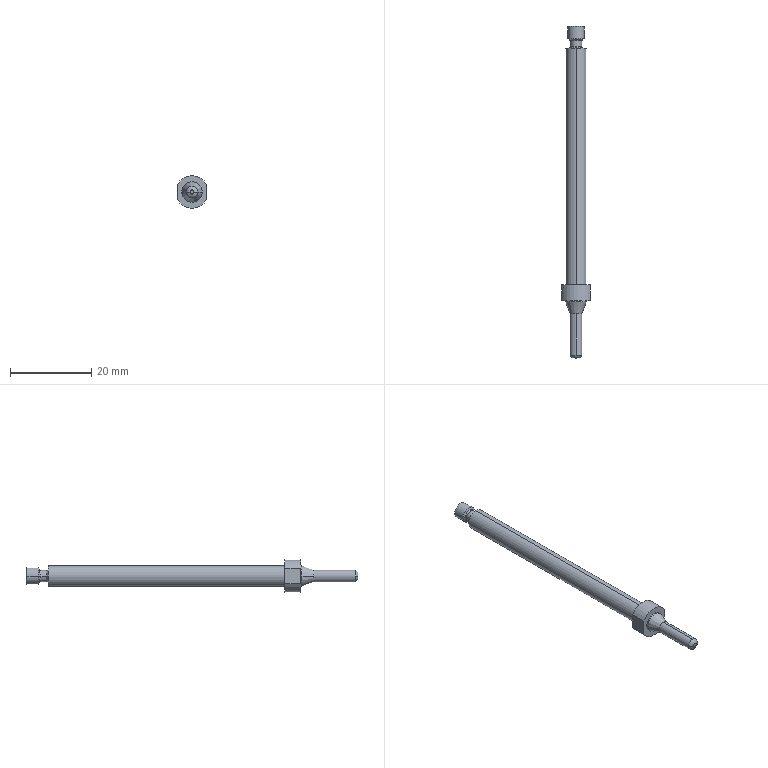Part | NX | 1 solid | 34 faces | box 7 x 81.5 x 8 mm | volume 1494 mm3 | cylinder 14 | plane 8 | cone 6 | torus 6 | commonest cylinder face diameters 4 x4 5 x4 2.8 x2 2.9 x2 8 x2
STEP:
#1=CARTESIAN_POINT('',(-125.5,76.718,117.869));
#2=VERTEX_POINT('',#1);
#3=CARTESIAN_POINT('',(-124.5,76.718,117.869));
#4=VERTEX_POINT('',#3);
#5=CARTESIAN_POINT('',(-125.,76.718,117.869));
#6=DIRECTION('',(0.,1.,0.));
#7=DIRECTION('',(0.,0.,1.));
#8=AXIS2_PLACEMENT_3D('',#5,#6,#7);
#9=CIRCLE('',#8,0.5);
#10=EDGE_CURVE('',#2,#4,#9,.T.);
#11=ORIENTED_EDGE('',*,*,#10,.F.);
#12=CARTESIAN_POINT('',(-125.,76.718,117.869));
#13=DIRECTION('',(0.,1.,0.));
#14=DIRECTION('',(0.,0.,1.));
#15=AXIS2_PLACEMENT_3D('',#12,#13,#14);
#16=CIRCLE('',#15,0.5);
#17=EDGE_CURVE('',#4,#2,#16,.T.);
#18=ORIENTED_EDGE('',*,*,#17,.F.);
#19=EDGE_LOOP('',(#11,#18));
#20=FACE_BOUND('',#19,.T.);
#21=CARTESIAN_POINT('',(-125.,76.718,119.817));
#22=DIRECTION('',(0.,1.,0.));
#23=DIRECTION('',(1.,0.,0.));
#24=AXIS2_PLACEMENT_3D('',#21,#22,#23);
#25=PLANE('',#24);
#26=ADVANCED_FACE('',(#20),#25,.F.);
#27=CARTESIAN_POINT('',(-125.,87.581,119.319));
#28=VERTEX_POINT('',#27);
#29=CARTESIAN_POINT('',(-123.55,87.581,117.869));
#30=VERTEX_POINT('',#29);
#31=CARTESIAN_POINT('',(-125.,87.581,117.869));
#32=DIRECTION('',(0.,1.,0.));
#33=DIRECTION('',(1.,0.,0.));
#34=AXIS2_PLACEMENT_3D('',#31,#32,#33);
#35=CIRCLE('',#34,1.45);
#36=EDGE_CURVE('',#28,#30,#35,.T.);
#37=ORIENTED_EDGE('',*,*,#36,.F.);
#38=CARTESIAN_POINT('',(-125.,77.406,119.319));
#39=VERTEX_POINT('',#38);
#40=CARTESIAN_POINT('',(-125.,90.3,119.319));
#41=DIRECTION('',(0.,1.,0.));
#42=VECTOR('',#41,1000.);
#43=LINE('',#40,#42);
#44=EDGE_CURVE('',#28,#39,#43,.F.);
#45=ORIENTED_EDGE('',*,*,#44,.T.);
#46=CARTESIAN_POINT('',(-123.55,77.406,117.869));
#47=VERTEX_POINT('',#46);
#48=CARTESIAN_POINT('',(-125.,77.406,117.869));
#49=DIRECTION('',(0.,1.,0.));
#50=DIRECTION('',(1.,0.,0.));
#51=AXIS2_PLACEMENT_3D('',#48,#49,#50);
#52=CIRCLE('',#51,1.45);
#53=EDGE_CURVE('',#39,#47,#52,.T.);
#54=ORIENTED_EDGE('',*,*,#53,.T.);
#55=CARTESIAN_POINT('',(-125.,77.406,116.419));
#56=VERTEX_POINT('',#55);
#57=CARTESIAN_POINT('',(-125.,77.406,117.869));
#58=DIRECTION('',(0.,1.,0.));
#59=DIRECTION('',(1.,0.,0.));
#60=AXIS2_PLACEMENT_3D('',#57,#58,#59);
#61=CIRCLE('',#60,1.45);
#62=EDGE_CURVE('',#47,#56,#61,.T.);
#63=ORIENTED_EDGE('',*,*,#62,.T.);
#64=CARTESIAN_POINT('',(-125.,87.581,116.419));
#65=VERTEX_POINT('',#64);
#66=CARTESIAN_POINT('',(-125.,90.3,116.419));
#67=DIRECTION('',(0.,1.,0.));
#68=VECTOR('',#67,1000.);
#69=LINE('',#66,#68);
#70=EDGE_CURVE('',#65,#56,#69,.F.);
#71=ORIENTED_EDGE('',*,*,#70,.F.);
#72=CARTESIAN_POINT('',(-125.,87.581,117.869));
#73=DIRECTION('',(0.,1.,0.));
#74=DIRECTION('',(1.,0.,0.));
#75=AXIS2_PLACEMENT_3D('',#72,#73,#74);
#76=CIRCLE('',#75,1.45);
#77=EDGE_CURVE('',#30,#65,#76,.T.);
#78=ORIENTED_EDGE('',*,*,#77,.F.);
#79=EDGE_LOOP('',(#37,#45,#54,#63,#71,#78));
#80=FACE_BOUND('',#79,.T.);
#81=CARTESIAN_POINT('',(-125.,90.3,117.869));
#82=DIRECTION('',(0.,1.,0.));
#83=DIRECTION('',(0.,0.,1.));
#84=AXIS2_PLACEMENT_3D('',#81,#82,#83);
#85=CYLINDRICAL_SURFACE('',#84,1.45);
#86=ADVANCED_FACE('',(#80),#85,.T.);
#87=CARTESIAN_POINT('',(-127.5,90.466,117.869));
#88=VERTEX_POINT('',#87);
#89=CARTESIAN_POINT('',(-125.,90.466,120.369));
#90=VERTEX_POINT('',#89);
#91=CARTESIAN_POINT('',(-125.,90.466,117.869));
#92=DIRECTION('',(0.,1.,0.));
#93=DIRECTION('',(0.,0.,1.));
#94=AXIS2_PLACEMENT_3D('',#91,#92,#93);
#95=CIRCLE('',#94,2.5);
#96=EDGE_CURVE('',#88,#90,#95,.T.);
#97=ORIENTED_EDGE('',*,*,#96,.F.);
#98=CARTESIAN_POINT('',(-126.45,87.581,117.869));
#99=VERTEX_POINT('',#98);
#100=CARTESIAN_POINT('',(-133.,105.577,117.869));
#101=DIRECTION('',(-0.342,0.9397,0.));
#102=VECTOR('',#101,1000.);
#103=LINE('',#100,#102);
#104=EDGE_CURVE('',#88,#99,#103,.F.);
#105=ORIENTED_EDGE('',*,*,#104,.T.);
#106=CARTESIAN_POINT('',(-125.,87.581,117.869));
#107=DIRECTION('',(0.,1.,0.));
#108=DIRECTION('',(1.,0.,0.));
#109=AXIS2_PLACEMENT_3D('',#106,#107,#108);
#110=CIRCLE('',#109,1.45);
#111=EDGE_CURVE('',#99,#28,#110,.T.);
#112=ORIENTED_EDGE('',*,*,#111,.T.);
#113=ORIENTED_EDGE('',*,*,#36,.T.);
#114=CARTESIAN_POINT('',(-122.5,90.466,117.869));
#115=VERTEX_POINT('',#114);
#116=CARTESIAN_POINT('',(-117.,105.577,117.869));
#117=DIRECTION('',(0.342,0.9397,0.));
#118=VECTOR('',#117,1000.);
#119=LINE('',#116,#118);
#120=EDGE_CURVE('',#115,#30,#119,.F.);
#121=ORIENTED_EDGE('',*,*,#120,.F.);
#122=CARTESIAN_POINT('',(-125.,90.466,117.869));
#123=DIRECTION('',(0.,1.,0.));
#124=DIRECTION('',(0.,0.,1.));
#125=AXIS2_PLACEMENT_3D('',#122,#123,#124);
#126=CIRCLE('',#125,2.5);
#127=EDGE_CURVE('',#90,#115,#126,.T.);
#128=ORIENTED_EDGE('',*,*,#127,.F.);
#129=EDGE_LOOP('',(#97,#105,#112,#113,#121,#128));
#130=FACE_BOUND('',#129,.T.);
#131=CARTESIAN_POINT('',(-125.,105.577,117.869));
#132=DIRECTION('',(0.,1.,0.));
#133=DIRECTION('',(1.,0.,0.));
#134=AXIS2_PLACEMENT_3D('',#131,#132,#133);
#135=CONICAL_SURFACE('',#134,8.,0.3491);
#136=ADVANCED_FACE('',(#130),#135,.T.);
#137=ORIENTED_EDGE('',*,*,#96,.T.);
#138=CARTESIAN_POINT('',(-125.,90.818,120.369));
#139=VERTEX_POINT('',#138);
#140=CARTESIAN_POINT('',(-125.,114.077,120.369));
#141=DIRECTION('',(0.,1.,0.));
#142=VECTOR('',#141,1000.);
#143=LINE('',#140,#142);
#144=EDGE_CURVE('',#90,#139,#143,.T.);
#145=ORIENTED_EDGE('',*,*,#144,.T.);
#146=CARTESIAN_POINT('',(-125.,90.818,115.369));
#147=VERTEX_POINT('',#146);
#148=CARTESIAN_POINT('',(-125.,90.818,117.869));
#149=DIRECTION('',(0.,1.,0.));
#150=DIRECTION('',(0.,0.,1.));
#151=AXIS2_PLACEMENT_3D('',#148,#149,#150);
#152=CIRCLE('',#151,2.5);
#153=EDGE_CURVE('',#147,#139,#152,.T.);
#154=ORIENTED_EDGE('',*,*,#153,.F.);
#155=CARTESIAN_POINT('',(-125.,90.466,115.369));
#156=VERTEX_POINT('',#155);
#157=CARTESIAN_POINT('',(-125.,114.077,115.369));
#158=DIRECTION('',(0.,1.,0.));
#159=VECTOR('',#158,1000.);
#160=LINE('',#157,#159);
#161=EDGE_CURVE('',#156,#147,#160,.T.);
#162=ORIENTED_EDGE('',*,*,#161,.F.);
#163=CARTESIAN_POINT('',(-125.,90.466,117.869));
#164=DIRECTION('',(0.,1.,0.));
#165=DIRECTION('',(0.,0.,1.));
#166=AXIS2_PLACEMENT_3D('',#163,#164,#165);
#167=CIRCLE('',#166,2.5);
#168=EDGE_CURVE('',#156,#88,#167,.T.);
#169=ORIENTED_EDGE('',*,*,#168,.T.);
#170=EDGE_LOOP('',(#137,#145,#154,#162,#169));
#171=FACE_BOUND('',#170,.T.);
#172=CARTESIAN_POINT('',(-125.,114.077,117.869));
#173=DIRECTION('',(0.,1.,0.));
#174=DIRECTION('',(0.,0.,1.));
#175=AXIS2_PLACEMENT_3D('',#172,#173,#174);
#176=CYLINDRICAL_SURFACE('',#175,2.5);
#177=ADVANCED_FACE('',(#171),#176,.T.);
#178=CARTESIAN_POINT('',(-121.5,94.718,119.805));
#179=VERTEX_POINT('',#178);
#180=CARTESIAN_POINT('',(-121.5,90.818,119.805));
#181=VERTEX_POINT('',#180);
#182=CARTESIAN_POINT('',(-121.5,94.718,119.805));
#183=DIRECTION('',(0.,-1.,0.));
#184=VECTOR('',#183,1000.);
#185=LINE('',#182,#184);
#186=EDGE_CURVE('',#179,#181,#185,.T.);
#187=ORIENTED_EDGE('',*,*,#186,.F.);
#188=CARTESIAN_POINT('',(-128.5,94.718,119.805));
#189=VERTEX_POINT('',#188);
#190=CARTESIAN_POINT('',(-125.,94.718,117.869));
#191=DIRECTION('',(0.,-1.,0.));
#192=DIRECTION('',(1.,0.,0.));
#193=AXIS2_PLACEMENT_3D('',#190,#191,#192);
#194=CIRCLE('',#193,4.);
#195=EDGE_CURVE('',#179,#189,#194,.T.);
#196=ORIENTED_EDGE('',*,*,#195,.T.);
#197=CARTESIAN_POINT('',(-128.5,90.818,119.805));
#198=VERTEX_POINT('',#197);
#199=CARTESIAN_POINT('',(-128.5,94.718,119.805));
#200=DIRECTION('',(0.,-1.,0.));
#201=VECTOR('',#200,1000.);
#202=LINE('',#199,#201);
#203=EDGE_CURVE('',#189,#198,#202,.T.);
#204=ORIENTED_EDGE('',*,*,#203,.T.);
#205=CARTESIAN_POINT('',(-125.,90.818,117.869));
#206=DIRECTION('',(0.,-1.,0.));
#207=DIRECTION('',(1.,0.,0.));
#208=AXIS2_PLACEMENT_3D('',#205,#206,#207);
#209=CIRCLE('',#208,4.);
#210=EDGE_CURVE('',#181,#198,#209,.T.);
#211=ORIENTED_EDGE('',*,*,#210,.F.);
#212=EDGE_LOOP('',(#187,#196,#204,#211));
#213=FACE_BOUND('',#212,.T.);
#214=CARTESIAN_POINT('',(-125.,94.718,117.869));
#215=DIRECTION('',(0.,-1.,0.));
#216=DIRECTION('',(1.,0.,0.));
#217=AXIS2_PLACEMENT_3D('',#214,#215,#216);
#218=CYLINDRICAL_SURFACE('',#217,4.);
#219=ADVANCED_FACE('',(#213),#218,.T.);
#220=CARTESIAN_POINT('',(-121.5,90.818,115.932));
#221=VERTEX_POINT('',#220);
#222=CARTESIAN_POINT('',(-121.5,90.818,0.));
#223=DIRECTION('',(0.,0.,-1.));
#224=VECTOR('',#223,1000.);
#225=LINE('',#222,#224);
#226=EDGE_CURVE('',#181,#221,#225,.T.);
#227=ORIENTED_EDGE('',*,*,#226,.F.);
#228=ORIENTED_EDGE('',*,*,#210,.T.);
#229=CARTESIAN_POINT('',(-128.5,90.818,115.932));
#230=VERTEX_POINT('',#229);
#231=CARTESIAN_POINT('',(-128.5,90.818,0.));
#232=DIRECTION('',(0.,0.,1.));
#233=VECTOR('',#232,1000.);
#234=LINE('',#231,#233);
#235=EDGE_CURVE('',#230,#198,#234,.T.);
#236=ORIENTED_EDGE('',*,*,#235,.F.);
#237=CARTESIAN_POINT('',(-125.,90.818,117.869));
#238=DIRECTION('',(0.,-1.,0.));
#239=DIRECTION('',(1.,0.,0.));
#240=AXIS2_PLACEMENT_3D('',#237,#238,#239);
#241=CIRCLE('',#240,4.);
#242=EDGE_CURVE('',#230,#221,#241,.T.);
#243=ORIENTED_EDGE('',*,*,#242,.T.);
#244=EDGE_LOOP('',(#227,#228,#236,#243));
#245=FACE_BOUND('',#244,.T.);
#246=ORIENTED_EDGE('',*,*,#153,.T.);
#247=CARTESIAN_POINT('',(-125.,90.818,117.869));
#248=DIRECTION('',(0.,1.,0.));
#249=DIRECTION('',(0.,0.,1.));
#250=AXIS2_PLACEMENT_3D('',#247,#248,#249);
#251=CIRCLE('',#250,2.5);
#252=EDGE_CURVE('',#139,#147,#251,.T.);
#253=ORIENTED_EDGE('',*,*,#252,.T.);
#254=EDGE_LOOP('',(#246,#253));
#255=FACE_BOUND('',#254,.T.);
#256=CARTESIAN_POINT('',(-123.871,90.818,119.664));
#257=DIRECTION('',(0.,-1.,0.));
#258=DIRECTION('',(0.,0.,-1.));
#259=AXIS2_PLACEMENT_3D('',#256,#257,#258);
#260=PLANE('',#259);
#261=ADVANCED_FACE('',(#245,#255),#260,.T.);
#262=CARTESIAN_POINT('',(-125.,152.718,120.369));
#263=VERTEX_POINT('',#262);
#264=CARTESIAN_POINT('',(-125.,152.718,115.369));
#265=VERTEX_POINT('',#264);
#266=CARTESIAN_POINT('',(-125.,152.718,117.869));
#267=DIRECTION('',(0.,1.,0.));
#268=DIRECTION('',(0.,0.,1.));
#269=AXIS2_PLACEMENT_3D('',#266,#267,#268);
#270=CIRCLE('',#269,2.5);
#271=EDGE_CURVE('',#263,#265,#270,.T.);
#272=ORIENTED_EDGE('',*,*,#271,.T.);
#273=CARTESIAN_POINT('',(-125.,152.718,117.869));
#274=DIRECTION('',(0.,1.,0.));
#275=DIRECTION('',(0.,0.,1.));
#276=AXIS2_PLACEMENT_3D('',#273,#274,#275);
#277=CIRCLE('',#276,2.5);
#278=EDGE_CURVE('',#265,#263,#277,.T.);
#279=ORIENTED_EDGE('',*,*,#278,.T.);
#280=EDGE_LOOP('',(#272,#279));
#281=FACE_BOUND('',#280,.T.);
#282=CARTESIAN_POINT('',(-123.,152.718,117.869));
#283=VERTEX_POINT('',#282);
#284=CARTESIAN_POINT('',(-127.,152.718,117.869));
#285=VERTEX_POINT('',#284);
#286=CARTESIAN_POINT('',(-125.,152.718,117.869));
#287=DIRECTION('',(0.,1.,0.));
#288=DIRECTION('',(-1.,0.,0.));
#289=AXIS2_PLACEMENT_3D('',#286,#287,#288);
#290=CIRCLE('',#289,2.);
#291=EDGE_CURVE('',#283,#285,#290,.T.);
#292=ORIENTED_EDGE('',*,*,#291,.F.);
#293=CARTESIAN_POINT('',(-125.,152.718,117.869));
#294=DIRECTION('',(0.,1.,0.));
#295=DIRECTION('',(-1.,0.,0.));
#296=AXIS2_PLACEMENT_3D('',#293,#294,#295);
#297=CIRCLE('',#296,2.);
#298=EDGE_CURVE('',#285,#283,#297,.T.);
#299=ORIENTED_EDGE('',*,*,#298,.F.);
#300=EDGE_LOOP('',(#292,#299));
#301=FACE_BOUND('',#300,.T.);
#302=CARTESIAN_POINT('',(-125.,152.718,123.869));
#303=DIRECTION('',(0.,1.,0.));
#304=DIRECTION('',(1.,0.,0.));
#305=AXIS2_PLACEMENT_3D('',#302,#303,#304);
#306=PLANE('',#305);
#307=ADVANCED_FACE('',(#281,#301),#306,.T.);
#308=ORIENTED_EDGE('',*,*,#53,.F.);
#309=CARTESIAN_POINT('',(-126.45,77.406,117.869));
#310=VERTEX_POINT('',#309);
#311=CARTESIAN_POINT('',(-125.,77.406,117.869));
#312=DIRECTION('',(0.,1.,0.));
#313=DIRECTION('',(1.,0.,0.));
#314=AXIS2_PLACEMENT_3D('',#311,#312,#313);
#315=CIRCLE('',#314,1.45);
#316=EDGE_CURVE('',#310,#39,#315,.T.);
#317=ORIENTED_EDGE('',*,*,#316,.F.);
#318=CARTESIAN_POINT('',(-125.5,77.718,117.869));
#319=DIRECTION('',(0.,0.,1.));
#320=DIRECTION('',(1.,0.,0.));
#321=AXIS2_PLACEMENT_3D('',#318,#319,#320);
#322=CIRCLE('',#321,1.);
#323=EDGE_CURVE('',#310,#2,#322,.T.);
#324=ORIENTED_EDGE('',*,*,#323,.T.);
#325=ORIENTED_EDGE('',*,*,#10,.T.);
#326=CARTESIAN_POINT('',(-124.5,77.718,117.869));
#327=DIRECTION('',(0.,0.,-1.));
#328=DIRECTION('',(-1.,0.,0.));
#329=AXIS2_PLACEMENT_3D('',#326,#327,#328);
#330=CIRCLE('',#329,1.);
#331=EDGE_CURVE('',#47,#4,#330,.T.);
#332=ORIENTED_EDGE('',*,*,#331,.F.);
#333=EDGE_LOOP('',(#308,#317,#324,#325,#332));
#334=FACE_BOUND('',#333,.T.);
#335=CARTESIAN_POINT('',(-125.,77.718,117.869));
#336=DIRECTION('',(0.,1.,0.));
#337=DIRECTION('',(1.,0.,0.));
#338=AXIS2_PLACEMENT_3D('',#335,#336,#337);
#339=DEGENERATE_TOROIDAL_SURFACE('',#338,0.5,1.,.T.);
#340=ADVANCED_FACE('',(#334),#339,.T.);
#341=ORIENTED_EDGE('',*,*,#271,.F.);
#342=CARTESIAN_POINT('',(-125.,94.718,120.369));
#343=VERTEX_POINT('',#342);
#344=CARTESIAN_POINT('',(-125.,114.077,120.369));
#345=DIRECTION('',(0.,1.,0.));
#346=VECTOR('',#345,1000.);
#347=LINE('',#344,#346);
#348=EDGE_CURVE('',#343,#263,#347,.T.);
#349=ORIENTED_EDGE('',*,*,#348,.F.);
#350=CARTESIAN_POINT('',(-125.,94.718,115.369));
#351=VERTEX_POINT('',#350);
#352=CARTESIAN_POINT('',(-125.,94.718,117.869));
#353=DIRECTION('',(0.,1.,0.));
#354=DIRECTION('',(0.,0.,1.));
#355=AXIS2_PLACEMENT_3D('',#352,#353,#354);
#356=CIRCLE('',#355,2.5);
#357=EDGE_CURVE('',#343,#351,#356,.T.);
#358=ORIENTED_EDGE('',*,*,#357,.T.);
#359=CARTESIAN_POINT('',(-125.,114.077,115.369));
#360=DIRECTION('',(0.,1.,0.));
#361=VECTOR('',#360,1000.);
#362=LINE('',#359,#361);
#363=EDGE_CURVE('',#351,#265,#362,.T.);
#364=ORIENTED_EDGE('',*,*,#363,.T.);
#365=EDGE_LOOP('',(#341,#349,#358,#364));
#366=FACE_BOUND('',#365,.T.);
#367=CARTESIAN_POINT('',(-125.,114.077,117.869));
#368=DIRECTION('',(0.,1.,0.));
#369=DIRECTION('',(0.,0.,1.));
#370=AXIS2_PLACEMENT_3D('',#367,#368,#369);
#371=CYLINDRICAL_SURFACE('',#370,2.5);
#372=ADVANCED_FACE('',(#366),#371,.T.);
#373=CARTESIAN_POINT('',(-128.5,94.718,115.932));
#374=VERTEX_POINT('',#373);
#375=CARTESIAN_POINT('',(-128.5,94.718,115.932));
#376=DIRECTION('',(0.,-1.,0.));
#377=VECTOR('',#376,1000.);
#378=LINE('',#375,#377);
#379=EDGE_CURVE('',#374,#230,#378,.T.);
#380=ORIENTED_EDGE('',*,*,#379,.F.);
#381=CARTESIAN_POINT('',(-121.5,94.718,115.932));
#382=VERTEX_POINT('',#381);
#383=CARTESIAN_POINT('',(-125.,94.718,117.869));
#384=DIRECTION('',(0.,-1.,0.));
#385=DIRECTION('',(1.,0.,0.));
#386=AXIS2_PLACEMENT_3D('',#383,#384,#385);
#387=CIRCLE('',#386,4.);
#388=EDGE_CURVE('',#374,#382,#387,.T.);
#389=ORIENTED_EDGE('',*,*,#388,.T.);
#390=CARTESIAN_POINT('',(-121.5,94.718,115.932));
#391=DIRECTION('',(0.,-1.,0.));
#392=VECTOR('',#391,1000.);
#393=LINE('',#390,#392);
#394=EDGE_CURVE('',#382,#221,#393,.T.);
#395=ORIENTED_EDGE('',*,*,#394,.T.);
#396=ORIENTED_EDGE('',*,*,#242,.F.);
#397=EDGE_LOOP('',(#380,#389,#395,#396));
#398=FACE_BOUND('',#397,.T.);
#399=CARTESIAN_POINT('',(-125.,94.718,117.869));
#400=DIRECTION('',(0.,-1.,0.));
#401=DIRECTION('',(1.,0.,0.));
#402=AXIS2_PLACEMENT_3D('',#399,#400,#401);
#403=CYLINDRICAL_SURFACE('',#402,4.);
#404=ADVANCED_FACE('',(#398),#403,.T.);
#405=CARTESIAN_POINT('',(-123.,152.818,117.869));
#406=VERTEX_POINT('',#405);
#407=CARTESIAN_POINT('',(-127.,152.818,117.869));
#408=VERTEX_POINT('',#407);
#409=CARTESIAN_POINT('',(-125.,152.818,117.869));
#410=DIRECTION('',(0.,1.,0.));
#411=DIRECTION('',(-1.,0.,0.));
#412=AXIS2_PLACEMENT_3D('',#409,#410,#411);
#413=CIRCLE('',#412,2.);
#414=EDGE_CURVE('',#406,#408,#413,.T.);
#415=ORIENTED_EDGE('',*,*,#414,.F.);
#416=CARTESIAN_POINT('',(-123.,152.718,117.869));
#417=DIRECTION('',(0.,1.,0.));
#418=VECTOR('',#417,1000.);
#419=LINE('',#416,#418);
#420=EDGE_CURVE('',#406,#283,#419,.F.);
#421=ORIENTED_EDGE('',*,*,#420,.T.);
#422=ORIENTED_EDGE('',*,*,#291,.T.);
#423=CARTESIAN_POINT('',(-127.,152.718,117.869));
#424=DIRECTION('',(0.,1.,0.));
#425=VECTOR('',#424,1000.);
#426=LINE('',#423,#425);
#427=EDGE_CURVE('',#408,#285,#426,.F.);
#428=ORIENTED_EDGE('',*,*,#427,.F.);
#429=EDGE_LOOP('',(#415,#421,#422,#428));
#430=FACE_BOUND('',#429,.T.);
#431=CARTESIAN_POINT('',(-125.,152.718,117.869));
#432=DIRECTION('',(0.,1.,0.));
#433=DIRECTION('',(-1.,0.,0.));
#434=AXIS2_PLACEMENT_3D('',#431,#432,#433);
#435=CYLINDRICAL_SURFACE('',#434,2.);
#436=ADVANCED_FACE('',(#430),#435,.T.);
#437=CARTESIAN_POINT('',(-123.35,158.218,117.869));
#438=VERTEX_POINT('',#437);
#439=CARTESIAN_POINT('',(-126.65,158.218,117.869));
#440=VERTEX_POINT('',#439);
#441=CARTESIAN_POINT('',(-125.,158.218,117.869));
#442=DIRECTION('',(0.,-1.,0.));
#443=DIRECTION('',(-1.,0.,0.));
#444=AXIS2_PLACEMENT_3D('',#441,#442,#443);
#445=CIRCLE('',#444,1.65);
#446=EDGE_CURVE('',#438,#440,#445,.T.);
#447=ORIENTED_EDGE('',*,*,#446,.F.);
#448=CARTESIAN_POINT('',(-125.,158.218,117.869));
#449=DIRECTION('',(0.,-1.,0.));
#450=DIRECTION('',(-1.,0.,0.));
#451=AXIS2_PLACEMENT_3D('',#448,#449,#450);
#452=CIRCLE('',#451,1.65);
#453=EDGE_CURVE('',#440,#438,#452,.T.);
#454=ORIENTED_EDGE('',*,*,#453,.F.);
#455=EDGE_LOOP('',(#447,#454));
#456=FACE_BOUND('',#455,.T.);
#457=CARTESIAN_POINT('',(-125.101,158.218,118.376));
#458=DIRECTION('',(0.,1.,0.));
#459=DIRECTION('',(1.,0.,0.));
#460=AXIS2_PLACEMENT_3D('',#457,#458,#459);
#461=PLANE('',#460);
#462=ADVANCED_FACE('',(#456),#461,.T.);
#463=CARTESIAN_POINT('',(-123.,155.118,117.869));
#464=VERTEX_POINT('',#463);
#465=CARTESIAN_POINT('',(-127.,155.118,117.869));
#466=VERTEX_POINT('',#465);
#467=CARTESIAN_POINT('',(-125.,155.118,117.869));
#468=DIRECTION('',(0.,1.,0.));
#469=DIRECTION('',(1.,0.,0.));
#470=AXIS2_PLACEMENT_3D('',#467,#468,#469);
#471=CIRCLE('',#470,2.);
#472=EDGE_CURVE('',#464,#466,#471,.T.);
#473=ORIENTED_EDGE('',*,*,#472,.T.);
#474=CARTESIAN_POINT('',(-127.,158.016,117.869));
#475=VERTEX_POINT('',#474);
#476=CARTESIAN_POINT('',(-127.,152.718,117.869));
#477=DIRECTION('',(0.,1.,0.));
#478=VECTOR('',#477,1000.);
#479=LINE('',#476,#478);
#480=EDGE_CURVE('',#475,#466,#479,.F.);
#481=ORIENTED_EDGE('',*,*,#480,.F.);
#482=CARTESIAN_POINT('',(-123.,158.016,117.869));
#483=VERTEX_POINT('',#482);
#484=CARTESIAN_POINT('',(-125.,158.016,117.869));
#485=DIRECTION('',(0.,-1.,0.));
#486=DIRECTION('',(-1.,0.,0.));
#487=AXIS2_PLACEMENT_3D('',#484,#485,#486);
#488=CIRCLE('',#487,2.);
#489=EDGE_CURVE('',#475,#483,#488,.T.);
#490=ORIENTED_EDGE('',*,*,#489,.T.);
#491=CARTESIAN_POINT('',(-123.,152.718,117.869));
#492=DIRECTION('',(0.,1.,0.));
#493=VECTOR('',#492,1000.);
#494=LINE('',#491,#493);
#495=EDGE_CURVE('',#483,#464,#494,.F.);
#496=ORIENTED_EDGE('',*,*,#495,.T.);
#497=EDGE_LOOP('',(#473,#481,#490,#496));
#498=FACE_BOUND('',#497,.T.);
#499=CARTESIAN_POINT('',(-125.,152.718,117.869));
#500=DIRECTION('',(0.,1.,0.));
#501=DIRECTION('',(-1.,0.,0.));
#502=AXIS2_PLACEMENT_3D('',#499,#500,#501);
#503=CYLINDRICAL_SURFACE('',#502,2.);
#504=ADVANCED_FACE('',(#498),#503,.T.);
#505=ORIENTED_EDGE('',*,*,#414,.T.);
#506=CARTESIAN_POINT('',(-125.,152.818,117.869));
#507=DIRECTION('',(0.,1.,0.));
#508=DIRECTION('',(-1.,0.,0.));
#509=AXIS2_PLACEMENT_3D('',#506,#507,#508);
#510=CIRCLE('',#509,2.);
#511=EDGE_CURVE('',#408,#406,#510,.T.);
#512=ORIENTED_EDGE('',*,*,#511,.T.);
#513=EDGE_LOOP('',(#505,#512));
#514=FACE_BOUND('',#513,.T.);
#515=CARTESIAN_POINT('',(-123.2,152.818,117.869));
#516=VERTEX_POINT('',#515);
#517=CARTESIAN_POINT('',(-126.8,152.818,117.869));
#518=VERTEX_POINT('',#517);
#519=CARTESIAN_POINT('',(-125.,152.818,117.869));
#520=DIRECTION('',(0.,-1.,0.));
#521=DIRECTION('',(-1.,0.,0.));
#522=AXIS2_PLACEMENT_3D('',#519,#520,#521);
#523=CIRCLE('',#522,1.8);
#524=EDGE_CURVE('',#516,#518,#523,.T.);
#525=ORIENTED_EDGE('',*,*,#524,.T.);
#526=CARTESIAN_POINT('',(-125.,152.818,117.869));
#527=DIRECTION('',(0.,-1.,0.));
#528=DIRECTION('',(-1.,0.,0.));
#529=AXIS2_PLACEMENT_3D('',#526,#527,#528);
#530=CIRCLE('',#529,1.8);
#531=EDGE_CURVE('',#518,#516,#530,.T.);
#532=ORIENTED_EDGE('',*,*,#531,.T.);
#533=EDGE_LOOP('',(#525,#532));
#534=FACE_BOUND('',#533,.T.);
#535=CARTESIAN_POINT('',(-125.,152.818,117.869));
#536=DIRECTION('',(0.,-1.,0.));
#537=DIRECTION('',(0.,0.,-1.));
#538=AXIS2_PLACEMENT_3D('',#535,#536,#537);
#539=PLANE('',#538);
#540=ADVANCED_FACE('',(#514,#534),#539,.F.);
#541=CARTESIAN_POINT('',(-123.6,154.541,117.869));
#542=VERTEX_POINT('',#541);
#543=CARTESIAN_POINT('',(-126.4,154.541,117.869));
#544=VERTEX_POINT('',#543);
#545=CARTESIAN_POINT('',(-125.,154.541,117.869));
#546=DIRECTION('',(0.,-1.,0.));
#547=DIRECTION('',(-1.,0.,0.));
#548=AXIS2_PLACEMENT_3D('',#545,#546,#547);
#549=CIRCLE('',#548,1.4);
#550=EDGE_CURVE('',#542,#544,#549,.T.);
#551=ORIENTED_EDGE('',*,*,#550,.T.);
#552=CARTESIAN_POINT('',(-126.4,153.218,117.869));
#553=VERTEX_POINT('',#552);
#554=CARTESIAN_POINT('',(-126.4,158.218,117.869));
#555=DIRECTION('',(0.,-1.,0.));
#556=VECTOR('',#555,1000.);
#557=LINE('',#554,#556);
#558=EDGE_CURVE('',#553,#544,#557,.F.);
#559=ORIENTED_EDGE('',*,*,#558,.F.);
#560=CARTESIAN_POINT('',(-123.6,153.218,117.869));
#561=VERTEX_POINT('',#560);
#562=CARTESIAN_POINT('',(-125.,153.218,117.869));
#563=DIRECTION('',(0.,-1.,0.));
#564=DIRECTION('',(-1.,0.,0.));
#565=AXIS2_PLACEMENT_3D('',#562,#563,#564);
#566=CIRCLE('',#565,1.4);
#567=EDGE_CURVE('',#561,#553,#566,.T.);
#568=ORIENTED_EDGE('',*,*,#567,.F.);
#569=CARTESIAN_POINT('',(-123.6,158.218,117.869));
#570=DIRECTION('',(0.,-1.,0.));
#571=VECTOR('',#570,1000.);
#572=LINE('',#569,#571);
#573=EDGE_CURVE('',#561,#542,#572,.F.);
#574=ORIENTED_EDGE('',*,*,#573,.T.);
#575=EDGE_LOOP('',(#551,#559,#568,#574));
#576=FACE_BOUND('',#575,.T.);
#577=CARTESIAN_POINT('',(-125.,158.218,117.869));
#578=DIRECTION('',(0.,-1.,0.));
#579=DIRECTION('',(-1.,0.,0.));
#580=AXIS2_PLACEMENT_3D('',#577,#578,#579);
#581=CYLINDRICAL_SURFACE('',#580,1.4);
#582=ADVANCED_FACE('',(#576),#581,.T.);
#583=ORIENTED_EDGE('',*,*,#472,.F.);
#584=CARTESIAN_POINT('',(-123.4,154.887,117.869));
#585=VERTEX_POINT('',#584);
#586=CARTESIAN_POINT('',(-123.,155.118,117.869));
#587=DIRECTION('',(0.866,0.5,0.));
#588=VECTOR('',#587,1000.);
#589=LINE('',#586,#588);
#590=EDGE_CURVE('',#585,#464,#589,.T.);
#591=ORIENTED_EDGE('',*,*,#590,.F.);
#592=CARTESIAN_POINT('',(-126.6,154.887,117.869));
#593=VERTEX_POINT('',#592);
#594=CARTESIAN_POINT('',(-125.,154.887,117.869));
#595=DIRECTION('',(0.,-1.,0.));
#596=DIRECTION('',(-1.,0.,0.));
#597=AXIS2_PLACEMENT_3D('',#594,#595,#596);
#598=CIRCLE('',#597,1.6);
#599=EDGE_CURVE('',#593,#585,#598,.T.);
#600=ORIENTED_EDGE('',*,*,#599,.F.);
#601=CARTESIAN_POINT('',(-127.,155.118,117.869));
#602=DIRECTION('',(-0.866,0.5,0.));
#603=VECTOR('',#602,1000.);
#604=LINE('',#601,#603);
#605=EDGE_CURVE('',#593,#466,#604,.T.);
#606=ORIENTED_EDGE('',*,*,#605,.T.);
#607=EDGE_LOOP('',(#583,#591,#600,#606));
#608=FACE_BOUND('',#607,.T.);
#609=CARTESIAN_POINT('',(-125.,155.118,117.869));
#610=DIRECTION('',(0.,1.,0.));
#611=DIRECTION('',(1.,0.,0.));
#612=AXIS2_PLACEMENT_3D('',#609,#610,#611);
#613=CONICAL_SURFACE('',#612,2.,1.047);
#614=ADVANCED_FACE('',(#608),#613,.T.);
#615=ORIENTED_EDGE('',*,*,#446,.T.);
#616=CARTESIAN_POINT('',(-126.65,158.218,117.869));
#617=DIRECTION('',(-0.866,-0.5,0.));
#618=VECTOR('',#617,1000.);
#619=LINE('',#616,#618);
#620=EDGE_CURVE('',#475,#440,#619,.F.);
#621=ORIENTED_EDGE('',*,*,#620,.F.);
#622=CARTESIAN_POINT('',(-125.,158.016,117.869));
#623=DIRECTION('',(0.,-1.,0.));
#624=DIRECTION('',(-1.,0.,0.));
#625=AXIS2_PLACEMENT_3D('',#622,#623,#624);
#626=CIRCLE('',#625,2.);
#627=EDGE_CURVE('',#483,#475,#626,.T.);
#628=ORIENTED_EDGE('',*,*,#627,.F.);
#629=CARTESIAN_POINT('',(-123.35,158.218,117.869));
#630=DIRECTION('',(0.866,-0.5,0.));
#631=VECTOR('',#630,1000.);
#632=LINE('',#629,#631);
#633=EDGE_CURVE('',#483,#438,#632,.F.);
#634=ORIENTED_EDGE('',*,*,#633,.T.);
#635=EDGE_LOOP('',(#615,#621,#628,#634));
#636=FACE_BOUND('',#635,.T.);
#637=CARTESIAN_POINT('',(-125.,158.218,117.869));
#638=DIRECTION('',(0.,-1.,0.));
#639=DIRECTION('',(-1.,0.,0.));
#640=AXIS2_PLACEMENT_3D('',#637,#638,#639);
#641=CONICAL_SURFACE('',#640,1.65,1.047);
#642=ADVANCED_FACE('',(#636),#641,.T.);
#643=ORIENTED_EDGE('',*,*,#550,.F.);
#644=CARTESIAN_POINT('',(-123.2,154.541,117.869));
#645=DIRECTION('',(0.,0.,1.));
#646=DIRECTION('',(1.,0.,0.));
#647=AXIS2_PLACEMENT_3D('',#644,#645,#646);
#648=CIRCLE('',#647,0.4);
#649=EDGE_CURVE('',#542,#585,#648,.F.);
#650=ORIENTED_EDGE('',*,*,#649,.T.);
#651=CARTESIAN_POINT('',(-125.,154.887,117.869));
#652=DIRECTION('',(0.,-1.,0.));
#653=DIRECTION('',(-1.,0.,0.));
#654=AXIS2_PLACEMENT_3D('',#651,#652,#653);
#655=CIRCLE('',#654,1.6);
#656=EDGE_CURVE('',#585,#593,#655,.T.);
#657=ORIENTED_EDGE('',*,*,#656,.T.);
#658=CARTESIAN_POINT('',(-126.8,154.541,117.869));
#659=DIRECTION('',(0.,0.,-1.));
#660=DIRECTION('',(-1.,0.,0.));
#661=AXIS2_PLACEMENT_3D('',#658,#659,#660);
#662=CIRCLE('',#661,0.4);
#663=EDGE_CURVE('',#544,#593,#662,.F.);
#664=ORIENTED_EDGE('',*,*,#663,.F.);
#665=EDGE_LOOP('',(#643,#650,#657,#664));
#666=FACE_BOUND('',#665,.T.);
#667=CARTESIAN_POINT('',(-125.,154.541,117.869));
#668=DIRECTION('',(0.,-1.,0.));
#669=DIRECTION('',(-1.,0.,0.));
#670=AXIS2_PLACEMENT_3D('',#667,#668,#669);
#671=TOROIDAL_SURFACE('',#670,1.8,0.4);
#672=ADVANCED_FACE('',(#666),#671,.F.);
#673=ORIENTED_EDGE('',*,*,#567,.T.);
#674=CARTESIAN_POINT('',(-126.8,153.218,117.869));
#675=DIRECTION('',(0.,0.,-1.));
#676=DIRECTION('',(-1.,0.,0.));
#677=AXIS2_PLACEMENT_3D('',#674,#675,#676);
#678=CIRCLE('',#677,0.4);
#679=EDGE_CURVE('',#518,#553,#678,.F.);
#680=ORIENTED_EDGE('',*,*,#679,.F.);
#681=ORIENTED_EDGE('',*,*,#524,.F.);
#682=CARTESIAN_POINT('',(-123.2,153.218,117.869));
#683=DIRECTION('',(0.,0.,1.));
#684=DIRECTION('',(1.,0.,0.));
#685=AXIS2_PLACEMENT_3D('',#682,#683,#684);
#686=CIRCLE('',#685,0.4);
#687=EDGE_CURVE('',#516,#561,#686,.F.);
#688=ORIENTED_EDGE('',*,*,#687,.T.);
#689=EDGE_LOOP('',(#673,#680,#681,#688));
#690=FACE_BOUND('',#689,.T.);
#691=CARTESIAN_POINT('',(-125.,153.218,117.869));
#692=DIRECTION('',(0.,-1.,0.));
#693=DIRECTION('',(-1.,0.,0.));
#694=AXIS2_PLACEMENT_3D('',#691,#692,#693);
#695=TOROIDAL_SURFACE('',#694,1.8,0.4);
#696=ADVANCED_FACE('',(#690),#695,.F.);
#697=CARTESIAN_POINT('',(-128.5,94.718,0.));
#698=DIRECTION('',(0.,0.,1.));
#699=VECTOR('',#698,1000.);
#700=LINE('',#697,#699);
#701=EDGE_CURVE('',#374,#189,#700,.T.);
#702=ORIENTED_EDGE('',*,*,#701,.T.);
#703=ORIENTED_EDGE('',*,*,#195,.F.);
#704=CARTESIAN_POINT('',(-121.5,94.718,0.));
#705=DIRECTION('',(0.,0.,-1.));
#706=VECTOR('',#705,1000.);
#707=LINE('',#704,#706);
#708=EDGE_CURVE('',#179,#382,#707,.T.);
#709=ORIENTED_EDGE('',*,*,#708,.T.);
#710=ORIENTED_EDGE('',*,*,#388,.F.);
#711=EDGE_LOOP('',(#702,#703,#709,#710));
#712=FACE_BOUND('',#711,.T.);
#713=CARTESIAN_POINT('',(-125.,94.718,117.869));
#714=DIRECTION('',(0.,1.,0.));
#715=DIRECTION('',(0.,0.,1.));
#716=AXIS2_PLACEMENT_3D('',#713,#714,#715);
#717=CIRCLE('',#716,2.5);
#718=EDGE_CURVE('',#351,#343,#717,.T.);
#719=ORIENTED_EDGE('',*,*,#718,.F.);
#720=ORIENTED_EDGE('',*,*,#357,.F.);
#721=EDGE_LOOP('',(#719,#720));
#722=FACE_BOUND('',#721,.T.);
#723=CARTESIAN_POINT('',(-123.871,94.718,119.664));
#724=DIRECTION('',(0.,-1.,0.));
#725=DIRECTION('',(0.,0.,-1.));
#726=AXIS2_PLACEMENT_3D('',#723,#724,#725);
#727=PLANE('',#726);
#728=ADVANCED_FACE('',(#712,#722),#727,.F.);
#729=ORIENTED_EDGE('',*,*,#226,.T.);
#730=ORIENTED_EDGE('',*,*,#394,.F.);
#731=ORIENTED_EDGE('',*,*,#708,.F.);
#732=ORIENTED_EDGE('',*,*,#186,.T.);
#733=EDGE_LOOP('',(#729,#730,#731,#732));
#734=FACE_BOUND('',#733,.T.);
#735=CARTESIAN_POINT('',(-121.5,87.818,113.069));
#736=DIRECTION('',(-1.,0.,0.));
#737=DIRECTION('',(0.,0.,1.));
#738=AXIS2_PLACEMENT_3D('',#735,#736,#737);
#739=PLANE('',#738);
#740=ADVANCED_FACE('',(#734),#739,.F.);
#741=ORIENTED_EDGE('',*,*,#379,.T.);
#742=ORIENTED_EDGE('',*,*,#235,.T.);
#743=ORIENTED_EDGE('',*,*,#203,.F.);
#744=ORIENTED_EDGE('',*,*,#701,.F.);
#745=EDGE_LOOP('',(#741,#742,#743,#744));
#746=FACE_BOUND('',#745,.T.);
#747=CARTESIAN_POINT('',(-128.5,94.718,113.069));
#748=DIRECTION('',(1.,0.,0.));
#749=DIRECTION('',(0.,1.,0.));
#750=AXIS2_PLACEMENT_3D('',#747,#748,#749);
#751=PLANE('',#750);
#752=ADVANCED_FACE('',(#746),#751,.F.);
#753=ORIENTED_EDGE('',*,*,#104,.F.);
#754=ORIENTED_EDGE('',*,*,#168,.F.);
#755=CARTESIAN_POINT('',(-125.,90.466,117.869));
#756=DIRECTION('',(0.,1.,0.));
#757=DIRECTION('',(0.,0.,1.));
#758=AXIS2_PLACEMENT_3D('',#755,#756,#757);
#759=CIRCLE('',#758,2.5);
#760=EDGE_CURVE('',#115,#156,#759,.T.);
#761=ORIENTED_EDGE('',*,*,#760,.F.);
#762=ORIENTED_EDGE('',*,*,#120,.T.);
#763=ORIENTED_EDGE('',*,*,#77,.T.);
#764=CARTESIAN_POINT('',(-125.,87.581,117.869));
#765=DIRECTION('',(0.,1.,0.));
#766=DIRECTION('',(1.,0.,0.));
#767=AXIS2_PLACEMENT_3D('',#764,#765,#766);
#768=CIRCLE('',#767,1.45);
#769=EDGE_CURVE('',#65,#99,#768,.T.);
#770=ORIENTED_EDGE('',*,*,#769,.T.);
#771=EDGE_LOOP('',(#753,#754,#761,#762,#763,#770));
#772=FACE_BOUND('',#771,.T.);
#773=CARTESIAN_POINT('',(-125.,105.577,117.869));
#774=DIRECTION('',(0.,1.,0.));
#775=DIRECTION('',(1.,0.,0.));
#776=AXIS2_PLACEMENT_3D('',#773,#774,#775);
#777=CONICAL_SURFACE('',#776,8.,0.3491);
#778=ADVANCED_FACE('',(#772),#777,.T.);
#779=ORIENTED_EDGE('',*,*,#718,.T.);
#780=ORIENTED_EDGE('',*,*,#348,.T.);
#781=ORIENTED_EDGE('',*,*,#278,.F.);
#782=ORIENTED_EDGE('',*,*,#363,.F.);
#783=EDGE_LOOP('',(#779,#780,#781,#782));
#784=FACE_BOUND('',#783,.T.);
#785=CARTESIAN_POINT('',(-125.,114.077,117.869));
#786=DIRECTION('',(0.,1.,0.));
#787=DIRECTION('',(0.,0.,1.));
#788=AXIS2_PLACEMENT_3D('',#785,#786,#787);
#789=CYLINDRICAL_SURFACE('',#788,2.5);
#790=ADVANCED_FACE('',(#784),#789,.T.);
#791=ORIENTED_EDGE('',*,*,#144,.F.);
#792=ORIENTED_EDGE('',*,*,#127,.T.);
#793=ORIENTED_EDGE('',*,*,#760,.T.);
#794=ORIENTED_EDGE('',*,*,#161,.T.);
#795=ORIENTED_EDGE('',*,*,#252,.F.);
#796=EDGE_LOOP('',(#791,#792,#793,#794,#795));
#797=FACE_BOUND('',#796,.T.);
#798=CARTESIAN_POINT('',(-125.,114.077,117.869));
#799=DIRECTION('',(0.,1.,0.));
#800=DIRECTION('',(0.,0.,1.));
#801=AXIS2_PLACEMENT_3D('',#798,#799,#800);
#802=CYLINDRICAL_SURFACE('',#801,2.5);
#803=ADVANCED_FACE('',(#797),#802,.T.);
#804=ORIENTED_EDGE('',*,*,#620,.T.);
#805=ORIENTED_EDGE('',*,*,#453,.T.);
#806=ORIENTED_EDGE('',*,*,#633,.F.);
#807=ORIENTED_EDGE('',*,*,#489,.F.);
#808=EDGE_LOOP('',(#804,#805,#806,#807));
#809=FACE_BOUND('',#808,.T.);
#810=CARTESIAN_POINT('',(-125.,158.218,117.869));
#811=DIRECTION('',(0.,-1.,0.));
#812=DIRECTION('',(-1.,0.,0.));
#813=AXIS2_PLACEMENT_3D('',#810,#811,#812);
#814=CONICAL_SURFACE('',#813,1.65,1.047);
#815=ADVANCED_FACE('',(#809),#814,.T.);
#816=ORIENTED_EDGE('',*,*,#656,.F.);
#817=ORIENTED_EDGE('',*,*,#590,.T.);
#818=CARTESIAN_POINT('',(-125.,155.118,117.869));
#819=DIRECTION('',(0.,1.,0.));
#820=DIRECTION('',(1.,0.,0.));
#821=AXIS2_PLACEMENT_3D('',#818,#819,#820);
#822=CIRCLE('',#821,2.);
#823=EDGE_CURVE('',#466,#464,#822,.T.);
#824=ORIENTED_EDGE('',*,*,#823,.F.);
#825=ORIENTED_EDGE('',*,*,#605,.F.);
#826=EDGE_LOOP('',(#816,#817,#824,#825));
#827=FACE_BOUND('',#826,.T.);
#828=CARTESIAN_POINT('',(-125.,155.118,117.869));
#829=DIRECTION('',(0.,1.,0.));
#830=DIRECTION('',(1.,0.,0.));
#831=AXIS2_PLACEMENT_3D('',#828,#829,#830);
#832=CONICAL_SURFACE('',#831,2.,1.047);
#833=ADVANCED_FACE('',(#827),#832,.T.);
#834=ORIENTED_EDGE('',*,*,#70,.T.);
#835=CARTESIAN_POINT('',(-125.,77.406,117.869));
#836=DIRECTION('',(0.,1.,0.));
#837=DIRECTION('',(1.,0.,0.));
#838=AXIS2_PLACEMENT_3D('',#835,#836,#837);
#839=CIRCLE('',#838,1.45);
#840=EDGE_CURVE('',#56,#310,#839,.T.);
#841=ORIENTED_EDGE('',*,*,#840,.T.);
#842=ORIENTED_EDGE('',*,*,#316,.T.);
#843=ORIENTED_EDGE('',*,*,#44,.F.);
#844=ORIENTED_EDGE('',*,*,#111,.F.);
#845=ORIENTED_EDGE('',*,*,#769,.F.);
#846=EDGE_LOOP('',(#834,#841,#842,#843,#844,#845));
#847=FACE_BOUND('',#846,.T.);
#848=CARTESIAN_POINT('',(-125.,90.3,117.869));
#849=DIRECTION('',(0.,1.,0.));
#850=DIRECTION('',(0.,0.,1.));
#851=AXIS2_PLACEMENT_3D('',#848,#849,#850);
#852=CYLINDRICAL_SURFACE('',#851,1.45);
#853=ADVANCED_FACE('',(#847),#852,.T.);
#854=ORIENTED_EDGE('',*,*,#627,.T.);
#855=ORIENTED_EDGE('',*,*,#480,.T.);
#856=ORIENTED_EDGE('',*,*,#823,.T.);
#857=ORIENTED_EDGE('',*,*,#495,.F.);
#858=EDGE_LOOP('',(#854,#855,#856,#857));
#859=FACE_BOUND('',#858,.T.);
#860=CARTESIAN_POINT('',(-125.,152.718,117.869));
#861=DIRECTION('',(0.,1.,0.));
#862=DIRECTION('',(-1.,0.,0.));
#863=AXIS2_PLACEMENT_3D('',#860,#861,#862);
#864=CYLINDRICAL_SURFACE('',#863,2.);
#865=ADVANCED_FACE('',(#859),#864,.T.);
#866=ORIENTED_EDGE('',*,*,#558,.T.);
#867=CARTESIAN_POINT('',(-125.,154.541,117.869));
#868=DIRECTION('',(0.,-1.,0.));
#869=DIRECTION('',(-1.,0.,0.));
#870=AXIS2_PLACEMENT_3D('',#867,#868,#869);
#871=CIRCLE('',#870,1.4);
#872=EDGE_CURVE('',#544,#542,#871,.T.);
#873=ORIENTED_EDGE('',*,*,#872,.T.);
#874=ORIENTED_EDGE('',*,*,#573,.F.);
#875=CARTESIAN_POINT('',(-125.,153.218,117.869));
#876=DIRECTION('',(0.,-1.,0.));
#877=DIRECTION('',(-1.,0.,0.));
#878=AXIS2_PLACEMENT_3D('',#875,#876,#877);
#879=CIRCLE('',#878,1.4);
#880=EDGE_CURVE('',#553,#561,#879,.T.);
#881=ORIENTED_EDGE('',*,*,#880,.F.);
#882=EDGE_LOOP('',(#866,#873,#874,#881));
#883=FACE_BOUND('',#882,.T.);
#884=CARTESIAN_POINT('',(-125.,158.218,117.869));
#885=DIRECTION('',(0.,-1.,0.));
#886=DIRECTION('',(-1.,0.,0.));
#887=AXIS2_PLACEMENT_3D('',#884,#885,#886);
#888=CYLINDRICAL_SURFACE('',#887,1.4);
#889=ADVANCED_FACE('',(#883),#888,.T.);
#890=ORIENTED_EDGE('',*,*,#427,.T.);
#891=ORIENTED_EDGE('',*,*,#298,.T.);
#892=ORIENTED_EDGE('',*,*,#420,.F.);
#893=ORIENTED_EDGE('',*,*,#511,.F.);
#894=EDGE_LOOP('',(#890,#891,#892,#893));
#895=FACE_BOUND('',#894,.T.);
#896=CARTESIAN_POINT('',(-125.,152.718,117.869));
#897=DIRECTION('',(0.,1.,0.));
#898=DIRECTION('',(-1.,0.,0.));
#899=AXIS2_PLACEMENT_3D('',#896,#897,#898);
#900=CYLINDRICAL_SURFACE('',#899,2.);
#901=ADVANCED_FACE('',(#895),#900,.T.);
#902=ORIENTED_EDGE('',*,*,#663,.T.);
#903=ORIENTED_EDGE('',*,*,#599,.T.);
#904=ORIENTED_EDGE('',*,*,#649,.F.);
#905=ORIENTED_EDGE('',*,*,#872,.F.);
#906=EDGE_LOOP('',(#902,#903,#904,#905));
#907=FACE_BOUND('',#906,.T.);
#908=CARTESIAN_POINT('',(-125.,154.541,117.869));
#909=DIRECTION('',(0.,-1.,0.));
#910=DIRECTION('',(-1.,0.,0.));
#911=AXIS2_PLACEMENT_3D('',#908,#909,#910);
#912=TOROIDAL_SURFACE('',#911,1.8,0.4);
#913=ADVANCED_FACE('',(#907),#912,.F.);
#914=ORIENTED_EDGE('',*,*,#331,.T.);
#915=ORIENTED_EDGE('',*,*,#17,.T.);
#916=ORIENTED_EDGE('',*,*,#323,.F.);
#917=ORIENTED_EDGE('',*,*,#840,.F.);
#918=ORIENTED_EDGE('',*,*,#62,.F.);
#919=EDGE_LOOP('',(#914,#915,#916,#917,#918));
#920=FACE_BOUND('',#919,.T.);
#921=CARTESIAN_POINT('',(-125.,77.718,117.869));
#922=DIRECTION('',(0.,1.,0.));
#923=DIRECTION('',(1.,0.,0.));
#924=AXIS2_PLACEMENT_3D('',#921,#922,#923);
#925=DEGENERATE_TOROIDAL_SURFACE('',#924,0.5,1.,.T.);
#926=ADVANCED_FACE('',(#920),#925,.T.);
#927=ORIENTED_EDGE('',*,*,#679,.T.);
#928=ORIENTED_EDGE('',*,*,#880,.T.);
#929=ORIENTED_EDGE('',*,*,#687,.F.);
#930=ORIENTED_EDGE('',*,*,#531,.F.);
#931=EDGE_LOOP('',(#927,#928,#929,#930));
#932=FACE_BOUND('',#931,.T.);
#933=CARTESIAN_POINT('',(-125.,153.218,117.869));
#934=DIRECTION('',(0.,-1.,0.));
#935=DIRECTION('',(-1.,0.,0.));
#936=AXIS2_PLACEMENT_3D('',#933,#934,#935);
#937=TOROIDAL_SURFACE('',#936,1.8,0.4);
#938=ADVANCED_FACE('',(#932),#937,.F.);
#939=CLOSED_SHELL('',(#26,#86,#136,#177,#219,#261,#307,#340,#372,#404,#436,#462,#504,#540,#582,#614,#642,#672,#696,#728,#740,#752,#778,#790,#803,#815,#833,#853,#865,#889,#901,#913,#926,#938));
#940=MANIFOLD_SOLID_BREP('',#939);
#941=(LENGTH_UNIT()NAMED_UNIT(*)SI_UNIT(.MILLI.,.METRE.));
#942=UNCERTAINTY_MEASURE_WITH_UNIT(LENGTH_MEASURE(0.00001),#941,'','');
#943=(NAMED_UNIT(*)PLANE_ANGLE_UNIT()SI_UNIT($,.RADIAN.));
#944=(NAMED_UNIT(*)SI_UNIT($,.STERADIAN.)SOLID_ANGLE_UNIT());
#945=(GEOMETRIC_REPRESENTATION_CONTEXT(3)GLOBAL_UNCERTAINTY_ASSIGNED_CONTEXT((#942))GLOBAL_UNIT_ASSIGNED_CONTEXT((#941,#943,#944))REPRESENTATION_CONTEXT('',''));
#946=ADVANCED_BREP_SHAPE_REPRESENTATION('',(#940),#945);